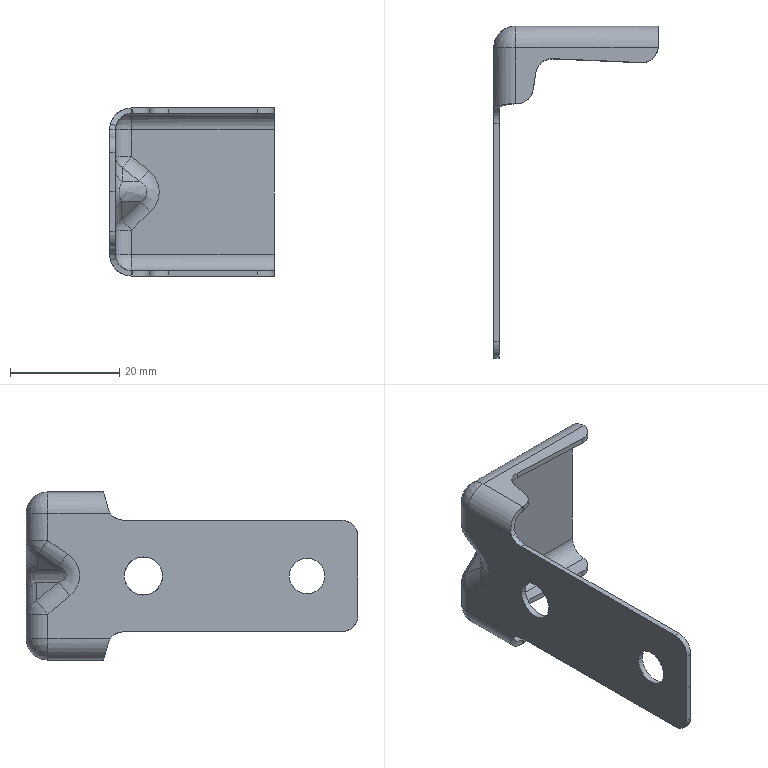Part | STEP file | FNA5401291 | 1 solid | 80 faces | box 30.161 x 60.798 x 30.791 mm | volume 2443 mm3 | cylinder 28 | spline 26 | plane 16 | sphere 8 | other 2 | commonest cylinder face diameters 6 x14 8 x10 6.5 x2 7 x2